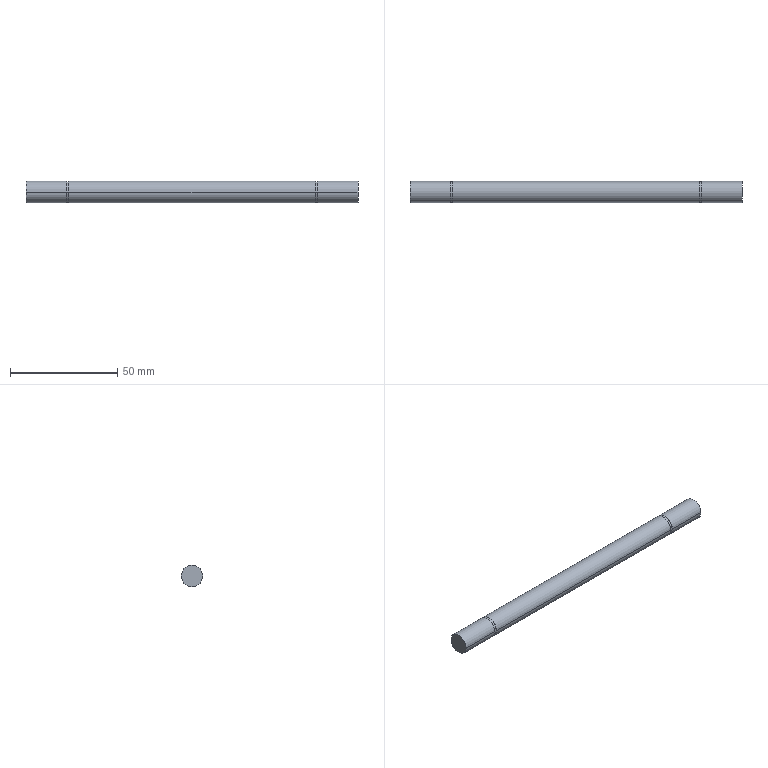Part | SolidWorks | features Revolution 1 | 1 solid | 16 faces | box 155 x 10 x 10 mm | volume 12160 mm3 | cylinder 10 | plane 6 | commonest cylinder face diameters 10 x6 9.6 x4
STEP:
#1=CARTESIAN_POINT('',(78.504,-7.107,0.));
#2=VERTEX_POINT('',#1);
#3=CARTESIAN_POINT('',(78.504,-17.107,0.));
#4=VERTEX_POINT('',#3);
#5=CARTESIAN_POINT('',(78.504,-12.107,0.));
#6=DIRECTION('',(1.,0.,0.));
#7=DIRECTION('',(0.,1.,0.));
#8=AXIS2_PLACEMENT_3D('',#5,#6,#7);
#9=CIRCLE('',#8,5.);
#10=EDGE_CURVE('',#2,#4,#9,.T.);
#11=ORIENTED_EDGE('',*,*,#10,.T.);
#12=CARTESIAN_POINT('',(97.404,-17.107,0.));
#13=VERTEX_POINT('',#12);
#14=CARTESIAN_POINT('',(97.404,-17.107,0.));
#15=DIRECTION('',(1.,0.,0.));
#16=VECTOR('',#15,1000.);
#17=LINE('',#14,#16);
#18=EDGE_CURVE('',#4,#13,#17,.T.);
#19=ORIENTED_EDGE('',*,*,#18,.T.);
#20=CARTESIAN_POINT('',(97.404,-7.107,0.));
#21=VERTEX_POINT('',#20);
#22=CARTESIAN_POINT('',(97.404,-12.107,0.));
#23=DIRECTION('',(1.,0.,0.));
#24=DIRECTION('',(0.,1.,0.));
#25=AXIS2_PLACEMENT_3D('',#22,#23,#24);
#26=CIRCLE('',#25,5.);
#27=EDGE_CURVE('',#21,#13,#26,.T.);
#28=ORIENTED_EDGE('',*,*,#27,.F.);
#29=CARTESIAN_POINT('',(97.404,-7.107,0.));
#30=DIRECTION('',(1.,0.,0.));
#31=VECTOR('',#30,1000.);
#32=LINE('',#29,#31);
#33=EDGE_CURVE('',#2,#21,#32,.T.);
#34=ORIENTED_EDGE('',*,*,#33,.F.);
#35=EDGE_LOOP('',(#11,#19,#28,#34));
#36=FACE_OUTER_BOUND('',#35,.T.);
#37=CARTESIAN_POINT('',(97.404,-12.107,0.));
#38=DIRECTION('',(1.,0.,0.));
#39=DIRECTION('',(0.,1.,0.));
#40=AXIS2_PLACEMENT_3D('',#37,#38,#39);
#41=CYLINDRICAL_SURFACE('',#40,5.);
#42=ADVANCED_FACE('',(#36),#41,.T.);
#43=CARTESIAN_POINT('',(77.404,-7.307,0.));
#44=VERTEX_POINT('',#43);
#45=CARTESIAN_POINT('',(77.404,-16.907,0.));
#46=VERTEX_POINT('',#45);
#47=CARTESIAN_POINT('',(77.404,-12.107,0.));
#48=DIRECTION('',(1.,0.,0.));
#49=DIRECTION('',(0.,1.,0.));
#50=AXIS2_PLACEMENT_3D('',#47,#48,#49);
#51=CIRCLE('',#50,4.8);
#52=EDGE_CURVE('',#44,#46,#51,.T.);
#53=ORIENTED_EDGE('',*,*,#52,.T.);
#54=CARTESIAN_POINT('',(78.504,-16.907,0.));
#55=VERTEX_POINT('',#54);
#56=CARTESIAN_POINT('',(97.404,-16.907,0.));
#57=DIRECTION('',(1.,0.,0.));
#58=VECTOR('',#57,1000.);
#59=LINE('',#56,#58);
#60=EDGE_CURVE('',#46,#55,#59,.T.);
#61=ORIENTED_EDGE('',*,*,#60,.T.);
#62=CARTESIAN_POINT('',(78.504,-7.307,0.));
#63=VERTEX_POINT('',#62);
#64=CARTESIAN_POINT('',(78.504,-12.107,0.));
#65=DIRECTION('',(1.,0.,0.));
#66=DIRECTION('',(0.,1.,0.));
#67=AXIS2_PLACEMENT_3D('',#64,#65,#66);
#68=CIRCLE('',#67,4.8);
#69=EDGE_CURVE('',#63,#55,#68,.T.);
#70=ORIENTED_EDGE('',*,*,#69,.F.);
#71=CARTESIAN_POINT('',(97.404,-7.307,0.));
#72=DIRECTION('',(1.,0.,0.));
#73=VECTOR('',#72,1000.);
#74=LINE('',#71,#73);
#75=EDGE_CURVE('',#44,#63,#74,.T.);
#76=ORIENTED_EDGE('',*,*,#75,.F.);
#77=EDGE_LOOP('',(#53,#61,#70,#76));
#78=FACE_OUTER_BOUND('',#77,.T.);
#79=CARTESIAN_POINT('',(97.404,-12.107,0.));
#80=DIRECTION('',(1.,0.,0.));
#81=DIRECTION('',(0.,1.,0.));
#82=AXIS2_PLACEMENT_3D('',#79,#80,#81);
#83=CYLINDRICAL_SURFACE('',#82,4.8);
#84=ADVANCED_FACE('',(#78),#83,.T.);
#85=CARTESIAN_POINT('',(-37.596,-7.107,0.));
#86=VERTEX_POINT('',#85);
#87=CARTESIAN_POINT('',(-37.596,-17.107,0.));
#88=VERTEX_POINT('',#87);
#89=CARTESIAN_POINT('',(-37.596,-12.107,0.));
#90=DIRECTION('',(1.,0.,0.));
#91=DIRECTION('',(0.,1.,0.));
#92=AXIS2_PLACEMENT_3D('',#89,#90,#91);
#93=CIRCLE('',#92,5.);
#94=EDGE_CURVE('',#86,#88,#93,.T.);
#95=ORIENTED_EDGE('',*,*,#94,.T.);
#96=CARTESIAN_POINT('',(77.404,-17.107,0.));
#97=VERTEX_POINT('',#96);
#98=CARTESIAN_POINT('',(97.404,-17.107,0.));
#99=DIRECTION('',(1.,0.,0.));
#100=VECTOR('',#99,1000.);
#101=LINE('',#98,#100);
#102=EDGE_CURVE('',#88,#97,#101,.T.);
#103=ORIENTED_EDGE('',*,*,#102,.T.);
#104=CARTESIAN_POINT('',(77.404,-7.107,0.));
#105=VERTEX_POINT('',#104);
#106=CARTESIAN_POINT('',(77.404,-12.107,0.));
#107=DIRECTION('',(1.,0.,0.));
#108=DIRECTION('',(0.,1.,0.));
#109=AXIS2_PLACEMENT_3D('',#106,#107,#108);
#110=CIRCLE('',#109,5.);
#111=EDGE_CURVE('',#105,#97,#110,.T.);
#112=ORIENTED_EDGE('',*,*,#111,.F.);
#113=CARTESIAN_POINT('',(97.404,-7.107,0.));
#114=DIRECTION('',(1.,0.,0.));
#115=VECTOR('',#114,1000.);
#116=LINE('',#113,#115);
#117=EDGE_CURVE('',#86,#105,#116,.T.);
#118=ORIENTED_EDGE('',*,*,#117,.F.);
#119=EDGE_LOOP('',(#95,#103,#112,#118));
#120=FACE_OUTER_BOUND('',#119,.T.);
#121=CARTESIAN_POINT('',(97.404,-12.107,0.));
#122=DIRECTION('',(1.,0.,0.));
#123=DIRECTION('',(0.,1.,0.));
#124=AXIS2_PLACEMENT_3D('',#121,#122,#123);
#125=CYLINDRICAL_SURFACE('',#124,5.);
#126=ADVANCED_FACE('',(#120),#125,.T.);
#127=CARTESIAN_POINT('',(-38.696,-7.307,0.));
#128=VERTEX_POINT('',#127);
#129=CARTESIAN_POINT('',(-38.696,-16.907,0.));
#130=VERTEX_POINT('',#129);
#131=CARTESIAN_POINT('',(-38.696,-12.107,0.));
#132=DIRECTION('',(1.,0.,0.));
#133=DIRECTION('',(0.,1.,0.));
#134=AXIS2_PLACEMENT_3D('',#131,#132,#133);
#135=CIRCLE('',#134,4.8);
#136=EDGE_CURVE('',#128,#130,#135,.T.);
#137=ORIENTED_EDGE('',*,*,#136,.T.);
#138=CARTESIAN_POINT('',(-37.596,-16.907,0.));
#139=VERTEX_POINT('',#138);
#140=CARTESIAN_POINT('',(97.404,-16.907,0.));
#141=DIRECTION('',(1.,0.,0.));
#142=VECTOR('',#141,1000.);
#143=LINE('',#140,#142);
#144=EDGE_CURVE('',#130,#139,#143,.T.);
#145=ORIENTED_EDGE('',*,*,#144,.T.);
#146=CARTESIAN_POINT('',(-37.596,-7.307,0.));
#147=VERTEX_POINT('',#146);
#148=CARTESIAN_POINT('',(-37.596,-12.107,0.));
#149=DIRECTION('',(1.,0.,0.));
#150=DIRECTION('',(0.,1.,0.));
#151=AXIS2_PLACEMENT_3D('',#148,#149,#150);
#152=CIRCLE('',#151,4.8);
#153=EDGE_CURVE('',#147,#139,#152,.T.);
#154=ORIENTED_EDGE('',*,*,#153,.F.);
#155=CARTESIAN_POINT('',(97.404,-7.307,0.));
#156=DIRECTION('',(1.,0.,0.));
#157=VECTOR('',#156,1000.);
#158=LINE('',#155,#157);
#159=EDGE_CURVE('',#128,#147,#158,.T.);
#160=ORIENTED_EDGE('',*,*,#159,.F.);
#161=EDGE_LOOP('',(#137,#145,#154,#160));
#162=FACE_OUTER_BOUND('',#161,.T.);
#163=CARTESIAN_POINT('',(97.404,-12.107,0.));
#164=DIRECTION('',(1.,0.,0.));
#165=DIRECTION('',(0.,1.,0.));
#166=AXIS2_PLACEMENT_3D('',#163,#164,#165);
#167=CYLINDRICAL_SURFACE('',#166,4.8);
#168=ADVANCED_FACE('',(#162),#167,.T.);
#169=CARTESIAN_POINT('',(-57.596,-7.107,0.));
#170=VERTEX_POINT('',#169);
#171=CARTESIAN_POINT('',(-57.596,-17.107,0.));
#172=VERTEX_POINT('',#171);
#173=CARTESIAN_POINT('',(-57.596,-12.107,0.));
#174=DIRECTION('',(1.,0.,0.));
#175=DIRECTION('',(0.,1.,0.));
#176=AXIS2_PLACEMENT_3D('',#173,#174,#175);
#177=CIRCLE('',#176,5.);
#178=EDGE_CURVE('',#170,#172,#177,.T.);
#179=ORIENTED_EDGE('',*,*,#178,.T.);
#180=CARTESIAN_POINT('',(-38.696,-17.107,0.));
#181=VERTEX_POINT('',#180);
#182=CARTESIAN_POINT('',(97.404,-17.107,0.));
#183=DIRECTION('',(1.,0.,0.));
#184=VECTOR('',#183,1000.);
#185=LINE('',#182,#184);
#186=EDGE_CURVE('',#172,#181,#185,.T.);
#187=ORIENTED_EDGE('',*,*,#186,.T.);
#188=CARTESIAN_POINT('',(-38.696,-7.107,0.));
#189=VERTEX_POINT('',#188);
#190=CARTESIAN_POINT('',(-38.696,-12.107,0.));
#191=DIRECTION('',(1.,0.,0.));
#192=DIRECTION('',(0.,1.,0.));
#193=AXIS2_PLACEMENT_3D('',#190,#191,#192);
#194=CIRCLE('',#193,5.);
#195=EDGE_CURVE('',#189,#181,#194,.T.);
#196=ORIENTED_EDGE('',*,*,#195,.F.);
#197=CARTESIAN_POINT('',(97.404,-7.107,0.));
#198=DIRECTION('',(1.,0.,0.));
#199=VECTOR('',#198,1000.);
#200=LINE('',#197,#199);
#201=EDGE_CURVE('',#170,#189,#200,.T.);
#202=ORIENTED_EDGE('',*,*,#201,.F.);
#203=EDGE_LOOP('',(#179,#187,#196,#202));
#204=FACE_OUTER_BOUND('',#203,.T.);
#205=CARTESIAN_POINT('',(97.404,-12.107,0.));
#206=DIRECTION('',(1.,0.,0.));
#207=DIRECTION('',(0.,1.,0.));
#208=AXIS2_PLACEMENT_3D('',#205,#206,#207);
#209=CYLINDRICAL_SURFACE('',#208,5.);
#210=ADVANCED_FACE('',(#204),#209,.T.);
#211=ORIENTED_EDGE('',*,*,#178,.F.);
#212=CARTESIAN_POINT('',(-57.596,-12.107,0.));
#213=DIRECTION('',(1.,0.,0.));
#214=DIRECTION('',(0.,1.,0.));
#215=AXIS2_PLACEMENT_3D('',#212,#213,#214);
#216=CIRCLE('',#215,5.);
#217=EDGE_CURVE('',#172,#170,#216,.T.);
#218=ORIENTED_EDGE('',*,*,#217,.F.);
#219=EDGE_LOOP('',(#211,#218));
#220=FACE_OUTER_BOUND('',#219,.T.);
#221=CARTESIAN_POINT('',(-57.596,-12.107,0.));
#222=DIRECTION('',(-1.,0.,0.));
#223=DIRECTION('',(0.,-1.,0.));
#224=AXIS2_PLACEMENT_3D('',#221,#222,#223);
#225=PLANE('',#224);
#226=ADVANCED_FACE('',(#220),#225,.T.);
#227=ORIENTED_EDGE('',*,*,#186,.F.);
#228=ORIENTED_EDGE('',*,*,#217,.T.);
#229=ORIENTED_EDGE('',*,*,#201,.T.);
#230=CARTESIAN_POINT('',(-38.696,-12.107,0.));
#231=DIRECTION('',(1.,0.,0.));
#232=DIRECTION('',(0.,1.,0.));
#233=AXIS2_PLACEMENT_3D('',#230,#231,#232);
#234=CIRCLE('',#233,5.);
#235=EDGE_CURVE('',#181,#189,#234,.T.);
#236=ORIENTED_EDGE('',*,*,#235,.F.);
#237=EDGE_LOOP('',(#227,#228,#229,#236));
#238=FACE_OUTER_BOUND('',#237,.T.);
#239=CARTESIAN_POINT('',(97.404,-12.107,0.));
#240=DIRECTION('',(1.,0.,0.));
#241=DIRECTION('',(0.,1.,0.));
#242=AXIS2_PLACEMENT_3D('',#239,#240,#241);
#243=CYLINDRICAL_SURFACE('',#242,5.);
#244=ADVANCED_FACE('',(#238),#243,.T.);
#245=ORIENTED_EDGE('',*,*,#195,.T.);
#246=ORIENTED_EDGE('',*,*,#235,.T.);
#247=EDGE_LOOP('',(#245,#246));
#248=FACE_OUTER_BOUND('',#247,.T.);
#249=ORIENTED_EDGE('',*,*,#136,.F.);
#250=CARTESIAN_POINT('',(-38.696,-12.107,0.));
#251=DIRECTION('',(1.,0.,0.));
#252=DIRECTION('',(0.,1.,0.));
#253=AXIS2_PLACEMENT_3D('',#250,#251,#252);
#254=CIRCLE('',#253,4.8);
#255=EDGE_CURVE('',#130,#128,#254,.T.);
#256=ORIENTED_EDGE('',*,*,#255,.F.);
#257=EDGE_LOOP('',(#249,#256));
#258=FACE_BOUND('',#257,.T.);
#259=CARTESIAN_POINT('',(-38.696,-7.107,0.));
#260=DIRECTION('',(1.,0.,0.));
#261=DIRECTION('',(0.,1.,0.));
#262=AXIS2_PLACEMENT_3D('',#259,#260,#261);
#263=PLANE('',#262);
#264=ADVANCED_FACE('',(#248,#258),#263,.T.);
#265=ORIENTED_EDGE('',*,*,#144,.F.);
#266=ORIENTED_EDGE('',*,*,#255,.T.);
#267=ORIENTED_EDGE('',*,*,#159,.T.);
#268=CARTESIAN_POINT('',(-37.596,-12.107,0.));
#269=DIRECTION('',(1.,0.,0.));
#270=DIRECTION('',(0.,1.,0.));
#271=AXIS2_PLACEMENT_3D('',#268,#269,#270);
#272=CIRCLE('',#271,4.8);
#273=EDGE_CURVE('',#139,#147,#272,.T.);
#274=ORIENTED_EDGE('',*,*,#273,.F.);
#275=EDGE_LOOP('',(#265,#266,#267,#274));
#276=FACE_OUTER_BOUND('',#275,.T.);
#277=CARTESIAN_POINT('',(97.404,-12.107,0.));
#278=DIRECTION('',(1.,0.,0.));
#279=DIRECTION('',(0.,1.,0.));
#280=AXIS2_PLACEMENT_3D('',#277,#278,#279);
#281=CYLINDRICAL_SURFACE('',#280,4.8);
#282=ADVANCED_FACE('',(#276),#281,.T.);
#283=ORIENTED_EDGE('',*,*,#153,.T.);
#284=ORIENTED_EDGE('',*,*,#273,.T.);
#285=EDGE_LOOP('',(#283,#284));
#286=FACE_BOUND('',#285,.T.);
#287=ORIENTED_EDGE('',*,*,#94,.F.);
#288=CARTESIAN_POINT('',(-37.596,-12.107,0.));
#289=DIRECTION('',(1.,0.,0.));
#290=DIRECTION('',(0.,1.,0.));
#291=AXIS2_PLACEMENT_3D('',#288,#289,#290);
#292=CIRCLE('',#291,5.);
#293=EDGE_CURVE('',#88,#86,#292,.T.);
#294=ORIENTED_EDGE('',*,*,#293,.F.);
#295=EDGE_LOOP('',(#287,#294));
#296=FACE_OUTER_BOUND('',#295,.T.);
#297=CARTESIAN_POINT('',(-37.596,-7.107,0.));
#298=DIRECTION('',(-1.,0.,0.));
#299=DIRECTION('',(0.,-1.,0.));
#300=AXIS2_PLACEMENT_3D('',#297,#298,#299);
#301=PLANE('',#300);
#302=ADVANCED_FACE('',(#286,#296),#301,.T.);
#303=ORIENTED_EDGE('',*,*,#102,.F.);
#304=ORIENTED_EDGE('',*,*,#293,.T.);
#305=ORIENTED_EDGE('',*,*,#117,.T.);
#306=CARTESIAN_POINT('',(77.404,-12.107,0.));
#307=DIRECTION('',(1.,0.,0.));
#308=DIRECTION('',(0.,1.,0.));
#309=AXIS2_PLACEMENT_3D('',#306,#307,#308);
#310=CIRCLE('',#309,5.);
#311=EDGE_CURVE('',#97,#105,#310,.T.);
#312=ORIENTED_EDGE('',*,*,#311,.F.);
#313=EDGE_LOOP('',(#303,#304,#305,#312));
#314=FACE_OUTER_BOUND('',#313,.T.);
#315=CARTESIAN_POINT('',(97.404,-12.107,0.));
#316=DIRECTION('',(1.,0.,0.));
#317=DIRECTION('',(0.,1.,0.));
#318=AXIS2_PLACEMENT_3D('',#315,#316,#317);
#319=CYLINDRICAL_SURFACE('',#318,5.);
#320=ADVANCED_FACE('',(#314),#319,.T.);
#321=ORIENTED_EDGE('',*,*,#111,.T.);
#322=ORIENTED_EDGE('',*,*,#311,.T.);
#323=EDGE_LOOP('',(#321,#322));
#324=FACE_OUTER_BOUND('',#323,.T.);
#325=ORIENTED_EDGE('',*,*,#52,.F.);
#326=CARTESIAN_POINT('',(77.404,-12.107,0.));
#327=DIRECTION('',(1.,0.,0.));
#328=DIRECTION('',(0.,1.,0.));
#329=AXIS2_PLACEMENT_3D('',#326,#327,#328);
#330=CIRCLE('',#329,4.8);
#331=EDGE_CURVE('',#46,#44,#330,.T.);
#332=ORIENTED_EDGE('',*,*,#331,.F.);
#333=EDGE_LOOP('',(#325,#332));
#334=FACE_BOUND('',#333,.T.);
#335=CARTESIAN_POINT('',(77.404,-7.107,0.));
#336=DIRECTION('',(1.,0.,0.));
#337=DIRECTION('',(0.,1.,0.));
#338=AXIS2_PLACEMENT_3D('',#335,#336,#337);
#339=PLANE('',#338);
#340=ADVANCED_FACE('',(#324,#334),#339,.T.);
#341=ORIENTED_EDGE('',*,*,#60,.F.);
#342=ORIENTED_EDGE('',*,*,#331,.T.);
#343=ORIENTED_EDGE('',*,*,#75,.T.);
#344=CARTESIAN_POINT('',(78.504,-12.107,0.));
#345=DIRECTION('',(1.,0.,0.));
#346=DIRECTION('',(0.,1.,0.));
#347=AXIS2_PLACEMENT_3D('',#344,#345,#346);
#348=CIRCLE('',#347,4.8);
#349=EDGE_CURVE('',#55,#63,#348,.T.);
#350=ORIENTED_EDGE('',*,*,#349,.F.);
#351=EDGE_LOOP('',(#341,#342,#343,#350));
#352=FACE_OUTER_BOUND('',#351,.T.);
#353=CARTESIAN_POINT('',(97.404,-12.107,0.));
#354=DIRECTION('',(1.,0.,0.));
#355=DIRECTION('',(0.,1.,0.));
#356=AXIS2_PLACEMENT_3D('',#353,#354,#355);
#357=CYLINDRICAL_SURFACE('',#356,4.8);
#358=ADVANCED_FACE('',(#352),#357,.T.);
#359=ORIENTED_EDGE('',*,*,#69,.T.);
#360=ORIENTED_EDGE('',*,*,#349,.T.);
#361=EDGE_LOOP('',(#359,#360));
#362=FACE_BOUND('',#361,.T.);
#363=ORIENTED_EDGE('',*,*,#10,.F.);
#364=CARTESIAN_POINT('',(78.504,-12.107,0.));
#365=DIRECTION('',(1.,0.,0.));
#366=DIRECTION('',(0.,1.,0.));
#367=AXIS2_PLACEMENT_3D('',#364,#365,#366);
#368=CIRCLE('',#367,5.);
#369=EDGE_CURVE('',#4,#2,#368,.T.);
#370=ORIENTED_EDGE('',*,*,#369,.F.);
#371=EDGE_LOOP('',(#363,#370));
#372=FACE_OUTER_BOUND('',#371,.T.);
#373=CARTESIAN_POINT('',(78.504,-7.107,0.));
#374=DIRECTION('',(-1.,0.,0.));
#375=DIRECTION('',(0.,-1.,0.));
#376=AXIS2_PLACEMENT_3D('',#373,#374,#375);
#377=PLANE('',#376);
#378=ADVANCED_FACE('',(#362,#372),#377,.T.);
#379=ORIENTED_EDGE('',*,*,#18,.F.);
#380=ORIENTED_EDGE('',*,*,#369,.T.);
#381=ORIENTED_EDGE('',*,*,#33,.T.);
#382=CARTESIAN_POINT('',(97.404,-12.107,0.));
#383=DIRECTION('',(1.,0.,0.));
#384=DIRECTION('',(0.,1.,0.));
#385=AXIS2_PLACEMENT_3D('',#382,#383,#384);
#386=CIRCLE('',#385,5.);
#387=EDGE_CURVE('',#13,#21,#386,.T.);
#388=ORIENTED_EDGE('',*,*,#387,.F.);
#389=EDGE_LOOP('',(#379,#380,#381,#388));
#390=FACE_OUTER_BOUND('',#389,.T.);
#391=CARTESIAN_POINT('',(97.404,-12.107,0.));
#392=DIRECTION('',(1.,0.,0.));
#393=DIRECTION('',(0.,1.,0.));
#394=AXIS2_PLACEMENT_3D('',#391,#392,#393);
#395=CYLINDRICAL_SURFACE('',#394,5.);
#396=ADVANCED_FACE('',(#390),#395,.T.);
#397=ORIENTED_EDGE('',*,*,#27,.T.);
#398=ORIENTED_EDGE('',*,*,#387,.T.);
#399=EDGE_LOOP('',(#397,#398));
#400=FACE_OUTER_BOUND('',#399,.T.);
#401=CARTESIAN_POINT('',(97.404,-7.107,0.));
#402=DIRECTION('',(1.,0.,0.));
#403=DIRECTION('',(0.,1.,0.));
#404=AXIS2_PLACEMENT_3D('',#401,#402,#403);
#405=PLANE('',#404);
#406=ADVANCED_FACE('',(#400),#405,.T.);
#407=CLOSED_SHELL('',(#42,#84,#126,#168,#210,#226,#244,#264,#282,#302,#320,#340,#358,#378,#396,#406));
#408=MANIFOLD_SOLID_BREP('',#407);
#409=CARTESIAN_POINT('',(0.,0.,0.));
#410=DIRECTION('',(0.,0.,1.));
#411=DIRECTION('',(1.,0.,0.));
#412=AXIS2_PLACEMENT_3D('',#409,#410,#411);
#413=(LENGTH_UNIT()NAMED_UNIT(*)SI_UNIT(.MILLI.,.METRE.));
#414=UNCERTAINTY_MEASURE_WITH_UNIT(LENGTH_MEASURE(0.00001),#413,'','');
#415=(NAMED_UNIT(*)PLANE_ANGLE_UNIT()SI_UNIT($,.RADIAN.));
#416=(NAMED_UNIT(*)SI_UNIT($,.STERADIAN.)SOLID_ANGLE_UNIT());
#417=(GEOMETRIC_REPRESENTATION_CONTEXT(3)GLOBAL_UNCERTAINTY_ASSIGNED_CONTEXT((#414))GLOBAL_UNIT_ASSIGNED_CONTEXT((#413,#415,#416))REPRESENTATION_CONTEXT('',''));
#418=ADVANCED_BREP_SHAPE_REPRESENTATION('',(#408,#412),#417);